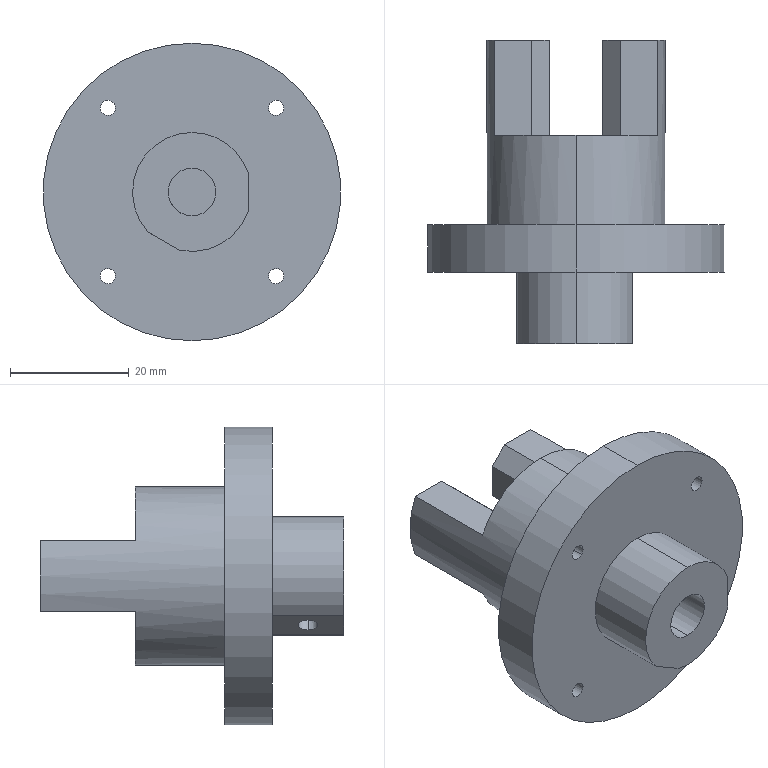Part | NX | features BREP 1 | 1 solid | 44 faces | box 50 x 51 x 50 mm | volume 32807 mm3 | cylinder 25 | plane 19 | commonest cylinder face diameters 2.5 x12 3.3 x4 20 x3 8 x2 30 x2 50 x2
STEP:
#1=CARTESIAN_POINT('',(14.122,12.,15.412));
#2=VERTEX_POINT('',#1);
#3=CARTESIAN_POINT('',(15.026,12.,15.026));
#4=VERTEX_POINT('',#3);
#5=CARTESIAN_POINT('',(14.122,12.,14.162));
#6=DIRECTION('',(0.,1.,0.));
#7=DIRECTION('',(0.,0.,1.));
#8=AXIS2_PLACEMENT_3D('',#5,#6,#7);
#9=CIRCLE('',#8,1.25);
#10=EDGE_CURVE('',#2,#4,#9,.T.);
#11=ORIENTED_EDGE('',*,*,#10,.F.);
#12=CARTESIAN_POINT('',(14.122,20.,15.412));
#13=VERTEX_POINT('',#12);
#14=CARTESIAN_POINT('',(14.122,20.,15.412));
#15=DIRECTION('',(0.,1.,0.));
#16=VECTOR('',#15,1000.);
#17=LINE('',#14,#16);
#18=EDGE_CURVE('',#2,#13,#17,.T.);
#19=ORIENTED_EDGE('',*,*,#18,.T.);
#20=CARTESIAN_POINT('',(15.026,20.,15.026));
#21=VERTEX_POINT('',#20);
#22=CARTESIAN_POINT('',(14.122,20.,14.162));
#23=DIRECTION('',(0.,1.,0.));
#24=DIRECTION('',(0.,0.,1.));
#25=AXIS2_PLACEMENT_3D('',#22,#23,#24);
#26=CIRCLE('',#25,1.25);
#27=EDGE_CURVE('',#13,#21,#26,.T.);
#28=ORIENTED_EDGE('',*,*,#27,.T.);
#29=CARTESIAN_POINT('',(15.026,15.75,15.026));
#30=DIRECTION('',(0.,1.,0.));
#31=VECTOR('',#30,1000.);
#32=LINE('',#29,#31);
#33=EDGE_CURVE('',#4,#21,#32,.T.);
#34=ORIENTED_EDGE('',*,*,#33,.F.);
#35=EDGE_LOOP('',(#11,#19,#28,#34));
#36=FACE_BOUND('',#35,.T.);
#37=CARTESIAN_POINT('',(14.122,20.,14.162));
#38=DIRECTION('',(0.,1.,0.));
#39=DIRECTION('',(0.,0.,-1.));
#40=AXIS2_PLACEMENT_3D('',#37,#38,#39);
#41=CYLINDRICAL_SURFACE('',#40,1.25);
#42=ADVANCED_FACE('',(#36),#41,.F.);
#43=CARTESIAN_POINT('',(-14.162,12.,-12.872));
#44=VERTEX_POINT('',#43);
#45=CARTESIAN_POINT('',(-13.258,12.,-13.258));
#46=VERTEX_POINT('',#45);
#47=CARTESIAN_POINT('',(-14.162,12.,-14.122));
#48=DIRECTION('',(0.,1.,0.));
#49=DIRECTION('',(0.,0.,1.));
#50=AXIS2_PLACEMENT_3D('',#47,#48,#49);
#51=CIRCLE('',#50,1.25);
#52=EDGE_CURVE('',#44,#46,#51,.T.);
#53=ORIENTED_EDGE('',*,*,#52,.F.);
#54=CARTESIAN_POINT('',(-14.162,20.,-12.872));
#55=VERTEX_POINT('',#54);
#56=CARTESIAN_POINT('',(-14.162,20.,-12.872));
#57=DIRECTION('',(0.,1.,0.));
#58=VECTOR('',#57,1000.);
#59=LINE('',#56,#58);
#60=EDGE_CURVE('',#44,#55,#59,.T.);
#61=ORIENTED_EDGE('',*,*,#60,.T.);
#62=CARTESIAN_POINT('',(-13.258,20.,-13.258));
#63=VERTEX_POINT('',#62);
#64=CARTESIAN_POINT('',(-14.162,20.,-14.122));
#65=DIRECTION('',(0.,1.,0.));
#66=DIRECTION('',(0.,0.,1.));
#67=AXIS2_PLACEMENT_3D('',#64,#65,#66);
#68=CIRCLE('',#67,1.25);
#69=EDGE_CURVE('',#55,#63,#68,.T.);
#70=ORIENTED_EDGE('',*,*,#69,.T.);
#71=CARTESIAN_POINT('',(-13.258,15.75,-13.258));
#72=DIRECTION('',(0.,1.,0.));
#73=VECTOR('',#72,1000.);
#74=LINE('',#71,#73);
#75=EDGE_CURVE('',#46,#63,#74,.T.);
#76=ORIENTED_EDGE('',*,*,#75,.F.);
#77=EDGE_LOOP('',(#53,#61,#70,#76));
#78=FACE_BOUND('',#77,.T.);
#79=CARTESIAN_POINT('',(-14.162,20.,-14.122));
#80=DIRECTION('',(0.,1.,0.));
#81=DIRECTION('',(0.,0.,-1.));
#82=AXIS2_PLACEMENT_3D('',#79,#80,#81);
#83=CYLINDRICAL_SURFACE('',#82,1.25);
#84=ADVANCED_FACE('',(#78),#83,.F.);
#85=CARTESIAN_POINT('',(14.162,12.,-12.872));
#86=VERTEX_POINT('',#85);
#87=CARTESIAN_POINT('',(15.026,12.,-15.026));
#88=VERTEX_POINT('',#87);
#89=CARTESIAN_POINT('',(14.162,12.,-14.122));
#90=DIRECTION('',(0.,1.,0.));
#91=DIRECTION('',(0.,0.,1.));
#92=AXIS2_PLACEMENT_3D('',#89,#90,#91);
#93=CIRCLE('',#92,1.25);
#94=EDGE_CURVE('',#86,#88,#93,.T.);
#95=ORIENTED_EDGE('',*,*,#94,.F.);
#96=CARTESIAN_POINT('',(14.162,20.,-12.872));
#97=VERTEX_POINT('',#96);
#98=CARTESIAN_POINT('',(14.162,20.,-12.872));
#99=DIRECTION('',(0.,1.,0.));
#100=VECTOR('',#99,1000.);
#101=LINE('',#98,#100);
#102=EDGE_CURVE('',#86,#97,#101,.T.);
#103=ORIENTED_EDGE('',*,*,#102,.T.);
#104=CARTESIAN_POINT('',(15.026,20.,-15.026));
#105=VERTEX_POINT('',#104);
#106=CARTESIAN_POINT('',(14.162,20.,-14.122));
#107=DIRECTION('',(0.,1.,0.));
#108=DIRECTION('',(0.,0.,1.));
#109=AXIS2_PLACEMENT_3D('',#106,#107,#108);
#110=CIRCLE('',#109,1.25);
#111=EDGE_CURVE('',#97,#105,#110,.T.);
#112=ORIENTED_EDGE('',*,*,#111,.T.);
#113=CARTESIAN_POINT('',(15.026,15.75,-15.026));
#114=DIRECTION('',(0.,-1.,0.));
#115=VECTOR('',#114,1000.);
#116=LINE('',#113,#115);
#117=EDGE_CURVE('',#105,#88,#116,.T.);
#118=ORIENTED_EDGE('',*,*,#117,.T.);
#119=EDGE_LOOP('',(#95,#103,#112,#118));
#120=FACE_BOUND('',#119,.T.);
#121=CARTESIAN_POINT('',(14.162,20.,-14.122));
#122=DIRECTION('',(0.,1.,0.));
#123=DIRECTION('',(0.,0.,-1.));
#124=AXIS2_PLACEMENT_3D('',#121,#122,#123);
#125=CYLINDRICAL_SURFACE('',#124,1.25);
#126=ADVANCED_FACE('',(#120),#125,.F.);
#127=CARTESIAN_POINT('',(-14.122,12.,15.412));
#128=VERTEX_POINT('',#127);
#129=CARTESIAN_POINT('',(-13.258,12.,13.258));
#130=VERTEX_POINT('',#129);
#131=CARTESIAN_POINT('',(-14.122,12.,14.162));
#132=DIRECTION('',(0.,1.,0.));
#133=DIRECTION('',(0.,0.,1.));
#134=AXIS2_PLACEMENT_3D('',#131,#132,#133);
#135=CIRCLE('',#134,1.25);
#136=EDGE_CURVE('',#128,#130,#135,.T.);
#137=ORIENTED_EDGE('',*,*,#136,.F.);
#138=CARTESIAN_POINT('',(-14.122,20.,15.412));
#139=VERTEX_POINT('',#138);
#140=CARTESIAN_POINT('',(-14.122,20.,15.412));
#141=DIRECTION('',(0.,1.,0.));
#142=VECTOR('',#141,1000.);
#143=LINE('',#140,#142);
#144=EDGE_CURVE('',#128,#139,#143,.T.);
#145=ORIENTED_EDGE('',*,*,#144,.T.);
#146=CARTESIAN_POINT('',(-13.258,20.,13.258));
#147=VERTEX_POINT('',#146);
#148=CARTESIAN_POINT('',(-14.122,20.,14.162));
#149=DIRECTION('',(0.,1.,0.));
#150=DIRECTION('',(0.,0.,1.));
#151=AXIS2_PLACEMENT_3D('',#148,#149,#150);
#152=CIRCLE('',#151,1.25);
#153=EDGE_CURVE('',#139,#147,#152,.T.);
#154=ORIENTED_EDGE('',*,*,#153,.T.);
#155=CARTESIAN_POINT('',(-13.258,15.75,13.258));
#156=DIRECTION('',(0.,1.,0.));
#157=VECTOR('',#156,1000.);
#158=LINE('',#155,#157);
#159=EDGE_CURVE('',#130,#147,#158,.T.);
#160=ORIENTED_EDGE('',*,*,#159,.F.);
#161=EDGE_LOOP('',(#137,#145,#154,#160));
#162=FACE_BOUND('',#161,.T.);
#163=CARTESIAN_POINT('',(-14.122,20.,14.162));
#164=DIRECTION('',(0.,1.,0.));
#165=DIRECTION('',(0.,0.,-1.));
#166=AXIS2_PLACEMENT_3D('',#163,#164,#165);
#167=CYLINDRICAL_SURFACE('',#166,1.25);
#168=ADVANCED_FACE('',(#162),#167,.F.);
#169=CARTESIAN_POINT('',(0.,20.,-15.));
#170=VERTEX_POINT('',#169);
#171=CARTESIAN_POINT('',(0.,20.,15.));
#172=VERTEX_POINT('',#171);
#173=CARTESIAN_POINT('',(0.,20.,0.));
#174=DIRECTION('',(0.,-1.,0.));
#175=DIRECTION('',(0.,0.,-1.));
#176=AXIS2_PLACEMENT_3D('',#173,#174,#175);
#177=CIRCLE('',#176,15.);
#178=EDGE_CURVE('',#170,#172,#177,.T.);
#179=ORIENTED_EDGE('',*,*,#178,.F.);
#180=CARTESIAN_POINT('',(0.,35.,-15.));
#181=VERTEX_POINT('',#180);
#182=CARTESIAN_POINT('',(0.,81.449,-15.));
#183=DIRECTION('',(0.,1.,0.));
#184=VECTOR('',#183,1000.);
#185=LINE('',#182,#184);
#186=EDGE_CURVE('',#170,#181,#185,.T.);
#187=ORIENTED_EDGE('',*,*,#186,.T.);
#188=CARTESIAN_POINT('',(13.748,35.,-6.));
#189=VERTEX_POINT('',#188);
#190=CARTESIAN_POINT('',(0.,35.,0.));
#191=DIRECTION('',(0.,1.,0.));
#192=DIRECTION('',(0.,0.,1.));
#193=AXIS2_PLACEMENT_3D('',#190,#191,#192);
#194=CIRCLE('',#193,15.);
#195=EDGE_CURVE('',#189,#181,#194,.T.);
#196=ORIENTED_EDGE('',*,*,#195,.F.);
#197=CARTESIAN_POINT('',(13.748,51.,-6.));
#198=VERTEX_POINT('',#197);
#199=CARTESIAN_POINT('',(13.748,81.449,-6.));
#200=DIRECTION('',(0.,1.,0.));
#201=VECTOR('',#200,1000.);
#202=LINE('',#199,#201);
#203=EDGE_CURVE('',#189,#198,#202,.T.);
#204=ORIENTED_EDGE('',*,*,#203,.T.);
#205=CARTESIAN_POINT('',(13.748,51.,6.));
#206=VERTEX_POINT('',#205);
#207=CARTESIAN_POINT('',(0.,51.,0.));
#208=DIRECTION('',(0.,1.,0.));
#209=DIRECTION('',(0.,0.,1.));
#210=AXIS2_PLACEMENT_3D('',#207,#208,#209);
#211=CIRCLE('',#210,15.);
#212=EDGE_CURVE('',#206,#198,#211,.T.);
#213=ORIENTED_EDGE('',*,*,#212,.F.);
#214=CARTESIAN_POINT('',(13.748,35.,6.));
#215=VERTEX_POINT('',#214);
#216=CARTESIAN_POINT('',(13.748,81.449,6.));
#217=DIRECTION('',(0.,-1.,0.));
#218=VECTOR('',#217,1000.);
#219=LINE('',#216,#218);
#220=EDGE_CURVE('',#206,#215,#219,.T.);
#221=ORIENTED_EDGE('',*,*,#220,.T.);
#222=CARTESIAN_POINT('',(0.,35.,15.));
#223=VERTEX_POINT('',#222);
#224=CARTESIAN_POINT('',(0.,35.,0.));
#225=DIRECTION('',(0.,1.,0.));
#226=DIRECTION('',(0.,0.,1.));
#227=AXIS2_PLACEMENT_3D('',#224,#225,#226);
#228=CIRCLE('',#227,15.);
#229=EDGE_CURVE('',#223,#215,#228,.T.);
#230=ORIENTED_EDGE('',*,*,#229,.F.);
#231=CARTESIAN_POINT('',(0.,81.449,15.));
#232=DIRECTION('',(0.,1.,0.));
#233=VECTOR('',#232,1000.);
#234=LINE('',#231,#233);
#235=EDGE_CURVE('',#172,#223,#234,.T.);
#236=ORIENTED_EDGE('',*,*,#235,.F.);
#237=EDGE_LOOP('',(#179,#187,#196,#204,#213,#221,#230,#236));
#238=FACE_BOUND('',#237,.T.);
#239=CARTESIAN_POINT('',(0.,81.449,0.));
#240=DIRECTION('',(0.,1.,0.));
#241=DIRECTION('',(0.,0.,-1.));
#242=AXIS2_PLACEMENT_3D('',#239,#240,#241);
#243=CYLINDRICAL_SURFACE('',#242,15.);
#244=ADVANCED_FACE('',(#238),#243,.T.);
#245=CARTESIAN_POINT('',(0.,20.,-25.));
#246=VERTEX_POINT('',#245);
#247=CARTESIAN_POINT('',(0.,20.,25.));
#248=VERTEX_POINT('',#247);
#249=CARTESIAN_POINT('',(0.,20.,0.));
#250=DIRECTION('',(0.,-1.,0.));
#251=DIRECTION('',(0.,0.,-1.));
#252=AXIS2_PLACEMENT_3D('',#249,#250,#251);
#253=CIRCLE('',#252,25.);
#254=EDGE_CURVE('',#246,#248,#253,.T.);
#255=ORIENTED_EDGE('',*,*,#254,.T.);
#256=CARTESIAN_POINT('',(0.,12.,25.));
#257=VERTEX_POINT('',#256);
#258=CARTESIAN_POINT('',(0.,20.,25.));
#259=DIRECTION('',(0.,-1.,0.));
#260=VECTOR('',#259,1000.);
#261=LINE('',#258,#260);
#262=EDGE_CURVE('',#257,#248,#261,.F.);
#263=ORIENTED_EDGE('',*,*,#262,.F.);
#264=CARTESIAN_POINT('',(0.,12.,-25.));
#265=VERTEX_POINT('',#264);
#266=CARTESIAN_POINT('',(0.,12.,0.));
#267=DIRECTION('',(0.,-1.,0.));
#268=DIRECTION('',(0.,0.,-1.));
#269=AXIS2_PLACEMENT_3D('',#266,#267,#268);
#270=CIRCLE('',#269,25.);
#271=EDGE_CURVE('',#265,#257,#270,.T.);
#272=ORIENTED_EDGE('',*,*,#271,.F.);
#273=CARTESIAN_POINT('',(0.,20.,-25.));
#274=DIRECTION('',(0.,-1.,0.));
#275=VECTOR('',#274,1000.);
#276=LINE('',#273,#275);
#277=EDGE_CURVE('',#265,#246,#276,.F.);
#278=ORIENTED_EDGE('',*,*,#277,.T.);
#279=EDGE_LOOP('',(#255,#263,#272,#278));
#280=FACE_BOUND('',#279,.T.);
#281=CARTESIAN_POINT('',(0.,20.,0.));
#282=DIRECTION('',(0.,-1.,0.));
#283=DIRECTION('',(0.,0.,1.));
#284=AXIS2_PLACEMENT_3D('',#281,#282,#283);
#285=CYLINDRICAL_SURFACE('',#284,25.);
#286=ADVANCED_FACE('',(#280),#285,.T.);
#287=CARTESIAN_POINT('',(-0.393,6.,-3.981));
#288=VERTEX_POINT('',#287);
#289=CARTESIAN_POINT('',(-3.251,6.,-2.331));
#290=VERTEX_POINT('',#289);
#291=CARTESIAN_POINT('',(-0.393,6.,-3.981));
#292=CARTESIAN_POINT('',(-0.393,5.559,-3.981));
#293=CARTESIAN_POINT('',(-0.7955,4.713,-3.963));
#294=CARTESIAN_POINT('',(-2.039,4.169,-3.539));
#295=CARTESIAN_POINT('',(-3.036,4.712,-2.67));
#296=CARTESIAN_POINT('',(-3.251,5.559,-2.331));
#297=CARTESIAN_POINT('',(-3.251,6.,-2.331));
#298=B_SPLINE_CURVE_WITH_KNOTS('',3,(#291,#292,#293,#294,#295,#296,#297),.UNSPECIFIED.,.F.,.F.,(4,1,1,1,4),(0.,0.001304,0.002607,0.003911,0.005215),.UNSPECIFIED.);
#299=EDGE_CURVE('',#288,#290,#298,.T.);
#300=ORIENTED_EDGE('',*,*,#299,.F.);
#301=CARTESIAN_POINT('',(-3.321,6.,-9.052));
#302=VERTEX_POINT('',#301);
#303=CARTESIAN_POINT('',(-3.571,6.,-9.485));
#304=DIRECTION('',(-0.5,0.,-0.866));
#305=VECTOR('',#304,1000.);
#306=LINE('',#303,#305);
#307=EDGE_CURVE('',#302,#288,#306,.F.);
#308=ORIENTED_EDGE('',*,*,#307,.F.);
#309=CARTESIAN_POINT('',(-6.179,6.,-7.402));
#310=VERTEX_POINT('',#309);
#311=CARTESIAN_POINT('',(-4.75,6.,-8.227));
#312=DIRECTION('',(-0.5,0.,-0.866));
#313=DIRECTION('',(0.866,0.,-0.5));
#314=AXIS2_PLACEMENT_3D('',#311,#312,#313);
#315=CIRCLE('',#314,1.65);
#316=EDGE_CURVE('',#302,#310,#315,.T.);
#317=ORIENTED_EDGE('',*,*,#316,.T.);
#318=CARTESIAN_POINT('',(-6.429,6.,-7.835));
#319=DIRECTION('',(-0.5,0.,-0.866));
#320=VECTOR('',#319,1000.);
#321=LINE('',#318,#320);
#322=EDGE_CURVE('',#310,#290,#321,.F.);
#323=ORIENTED_EDGE('',*,*,#322,.T.);
#324=EDGE_LOOP('',(#300,#308,#317,#323));
#325=FACE_BOUND('',#324,.T.);
#326=CARTESIAN_POINT('',(-5.,6.,-8.66));
#327=DIRECTION('',(-0.5,0.,-0.866));
#328=DIRECTION('',(0.866,0.,-0.5));
#329=AXIS2_PLACEMENT_3D('',#326,#327,#328);
#330=CYLINDRICAL_SURFACE('',#329,1.65);
#331=ADVANCED_FACE('',(#325),#330,.F.);
#332=CARTESIAN_POINT('',(3.644,6.,1.65));
#333=VERTEX_POINT('',#332);
#334=CARTESIAN_POINT('',(3.644,6.,-1.65));
#335=VERTEX_POINT('',#334);
#336=CARTESIAN_POINT('',(3.644,6.,1.65));
#337=CARTESIAN_POINT('',(3.644,5.559,1.65));
#338=CARTESIAN_POINT('',(3.83,4.713,1.293));
#339=CARTESIAN_POINT('',(4.085,4.169,0.003454));
#340=CARTESIAN_POINT('',(3.83,4.712,-1.294));
#341=CARTESIAN_POINT('',(3.644,5.559,-1.65));
#342=CARTESIAN_POINT('',(3.644,6.,-1.65));
#343=B_SPLINE_CURVE_WITH_KNOTS('',3,(#336,#337,#338,#339,#340,#341,#342),.UNSPECIFIED.,.F.,.F.,(4,1,1,1,4),(0.,0.001304,0.002607,0.003911,0.005215),.UNSPECIFIED.);
#344=EDGE_CURVE('',#333,#335,#343,.T.);
#345=ORIENTED_EDGE('',*,*,#344,.F.);
#346=CARTESIAN_POINT('',(9.5,6.,1.65));
#347=VERTEX_POINT('',#346);
#348=CARTESIAN_POINT('',(10.,6.,1.65));
#349=DIRECTION('',(1.,0.,0.));
#350=VECTOR('',#349,1000.);
#351=LINE('',#348,#350);
#352=EDGE_CURVE('',#347,#333,#351,.F.);
#353=ORIENTED_EDGE('',*,*,#352,.F.);
#354=CARTESIAN_POINT('',(9.5,6.,-1.65));
#355=VERTEX_POINT('',#354);
#356=CARTESIAN_POINT('',(9.5,6.,0.));
#357=DIRECTION('',(1.,0.,0.));
#358=DIRECTION('',(0.,0.,1.));
#359=AXIS2_PLACEMENT_3D('',#356,#357,#358);
#360=CIRCLE('',#359,1.65);
#361=EDGE_CURVE('',#347,#355,#360,.T.);
#362=ORIENTED_EDGE('',*,*,#361,.T.);
#363=CARTESIAN_POINT('',(10.,6.,-1.65));
#364=DIRECTION('',(1.,0.,0.));
#365=VECTOR('',#364,1000.);
#366=LINE('',#363,#365);
#367=EDGE_CURVE('',#355,#335,#366,.F.);
#368=ORIENTED_EDGE('',*,*,#367,.T.);
#369=EDGE_LOOP('',(#345,#353,#362,#368));
#370=FACE_BOUND('',#369,.T.);
#371=CARTESIAN_POINT('',(10.,6.,0.));
#372=DIRECTION('',(1.,0.,0.));
#373=DIRECTION('',(0.,0.,1.));
#374=AXIS2_PLACEMENT_3D('',#371,#372,#373);
#375=CYLINDRICAL_SURFACE('',#374,1.65);
#376=ADVANCED_FACE('',(#370),#375,.F.);
#377=CARTESIAN_POINT('',(-3.251,6.,-2.331));
#378=CARTESIAN_POINT('',(-3.251,6.441,-2.331));
#379=CARTESIAN_POINT('',(-3.034,7.287,-2.671));
#380=CARTESIAN_POINT('',(-2.045,7.831,-3.536));
#381=CARTESIAN_POINT('',(-0.7946,7.288,-3.964));
#382=CARTESIAN_POINT('',(-0.393,6.441,-3.981));
#383=CARTESIAN_POINT('',(-0.393,6.,-3.981));
#384=B_SPLINE_CURVE_WITH_KNOTS('',3,(#377,#378,#379,#380,#381,#382,#383),.UNSPECIFIED.,.F.,.F.,(4,1,1,1,4),(0.,0.001304,0.002607,0.003911,0.005215),.UNSPECIFIED.);
#385=EDGE_CURVE('',#290,#288,#384,.T.);
#386=ORIENTED_EDGE('',*,*,#385,.T.);
#387=ORIENTED_EDGE('',*,*,#299,.T.);
#388=EDGE_LOOP('',(#386,#387));
#389=FACE_BOUND('',#388,.T.);
#390=CARTESIAN_POINT('',(0.,11.,4.));
#391=VERTEX_POINT('',#390);
#392=CARTESIAN_POINT('',(0.,11.,-4.));
#393=VERTEX_POINT('',#392);
#394=CARTESIAN_POINT('',(0.,11.,0.));
#395=DIRECTION('',(0.,-1.,0.));
#396=DIRECTION('',(0.,0.,-1.));
#397=AXIS2_PLACEMENT_3D('',#394,#395,#396);
#398=CIRCLE('',#397,4.);
#399=EDGE_CURVE('',#391,#393,#398,.T.);
#400=ORIENTED_EDGE('',*,*,#399,.F.);
#401=CARTESIAN_POINT('',(0.,0.,4.));
#402=VERTEX_POINT('',#401);
#403=CARTESIAN_POINT('',(0.,11.,4.));
#404=DIRECTION('',(0.,-1.,0.));
#405=VECTOR('',#404,1000.);
#406=LINE('',#403,#405);
#407=EDGE_CURVE('',#402,#391,#406,.F.);
#408=ORIENTED_EDGE('',*,*,#407,.F.);
#409=CARTESIAN_POINT('',(0.,0.,-4.));
#410=VERTEX_POINT('',#409);
#411=CARTESIAN_POINT('',(0.,0.,0.));
#412=DIRECTION('',(0.,-1.,0.));
#413=DIRECTION('',(0.,0.,-1.));
#414=AXIS2_PLACEMENT_3D('',#411,#412,#413);
#415=CIRCLE('',#414,4.);
#416=EDGE_CURVE('',#402,#410,#415,.T.);
#417=ORIENTED_EDGE('',*,*,#416,.T.);
#418=CARTESIAN_POINT('',(0.,11.,-4.));
#419=DIRECTION('',(0.,-1.,0.));
#420=VECTOR('',#419,1000.);
#421=LINE('',#418,#420);
#422=EDGE_CURVE('',#410,#393,#421,.F.);
#423=ORIENTED_EDGE('',*,*,#422,.T.);
#424=EDGE_LOOP('',(#400,#408,#417,#423));
#425=FACE_BOUND('',#424,.T.);
#426=CARTESIAN_POINT('',(0.,11.,0.));
#427=DIRECTION('',(0.,-1.,0.));
#428=DIRECTION('',(0.,0.,1.));
#429=AXIS2_PLACEMENT_3D('',#426,#427,#428);
#430=CYLINDRICAL_SURFACE('',#429,4.);
#431=ADVANCED_FACE('',(#389,#425),#430,.F.);
#432=CARTESIAN_POINT('',(-7.454,0.,-6.666));
#433=VERTEX_POINT('',#432);
#434=CARTESIAN_POINT('',(0.,0.,10.));
#435=VERTEX_POINT('',#434);
#436=CARTESIAN_POINT('',(0.,0.,0.));
#437=DIRECTION('',(0.,1.,0.));
#438=DIRECTION('',(0.,0.,1.));
#439=AXIS2_PLACEMENT_3D('',#436,#437,#438);
#440=CIRCLE('',#439,10.);
#441=EDGE_CURVE('',#433,#435,#440,.T.);
#442=ORIENTED_EDGE('',*,*,#441,.T.);
#443=CARTESIAN_POINT('',(0.,12.,10.));
#444=VERTEX_POINT('',#443);
#445=CARTESIAN_POINT('',(0.,81.449,10.));
#446=DIRECTION('',(0.,1.,0.));
#447=VECTOR('',#446,1000.);
#448=LINE('',#445,#447);
#449=EDGE_CURVE('',#435,#444,#448,.T.);
#450=ORIENTED_EDGE('',*,*,#449,.T.);
#451=CARTESIAN_POINT('',(-7.454,12.,-6.666));
#452=VERTEX_POINT('',#451);
#453=CARTESIAN_POINT('',(0.,12.,0.));
#454=DIRECTION('',(0.,1.,0.));
#455=DIRECTION('',(0.,0.,1.));
#456=AXIS2_PLACEMENT_3D('',#453,#454,#455);
#457=CIRCLE('',#456,10.);
#458=EDGE_CURVE('',#452,#444,#457,.T.);
#459=ORIENTED_EDGE('',*,*,#458,.F.);
#460=CARTESIAN_POINT('',(-7.454,18.245,-6.666));
#461=DIRECTION('',(0.,-1.,0.));
#462=VECTOR('',#461,1000.);
#463=LINE('',#460,#462);
#464=EDGE_CURVE('',#452,#433,#463,.T.);
#465=ORIENTED_EDGE('',*,*,#464,.T.);
#466=EDGE_LOOP('',(#442,#450,#459,#465));
#467=FACE_BOUND('',#466,.T.);
#468=CARTESIAN_POINT('',(0.,81.449,0.));
#469=DIRECTION('',(0.,1.,0.));
#470=DIRECTION('',(0.,0.,-1.));
#471=AXIS2_PLACEMENT_3D('',#468,#469,#470);
#472=CYLINDRICAL_SURFACE('',#471,10.);
#473=ADVANCED_FACE('',(#467),#472,.T.);
#474=CARTESIAN_POINT('',(13.258,20.,13.258));
#475=VERTEX_POINT('',#474);
#476=CARTESIAN_POINT('',(14.122,20.,14.162));
#477=DIRECTION('',(0.,1.,0.));
#478=DIRECTION('',(0.,0.,1.));
#479=AXIS2_PLACEMENT_3D('',#476,#477,#478);
#480=CIRCLE('',#479,1.25);
#481=EDGE_CURVE('',#475,#13,#480,.T.);
#482=ORIENTED_EDGE('',*,*,#481,.F.);
#483=CARTESIAN_POINT('',(14.162,20.,14.122));
#484=DIRECTION('',(0.,1.,0.));
#485=DIRECTION('',(0.,0.,1.));
#486=AXIS2_PLACEMENT_3D('',#483,#484,#485);
#487=CIRCLE('',#486,1.25);
#488=EDGE_CURVE('',#21,#475,#487,.T.);
#489=ORIENTED_EDGE('',*,*,#488,.F.);
#490=ORIENTED_EDGE('',*,*,#27,.F.);
#491=EDGE_LOOP('',(#482,#489,#490));
#492=FACE_BOUND('',#491,.T.);
#493=CARTESIAN_POINT('',(-15.026,20.,15.026));
#494=VERTEX_POINT('',#493);
#495=CARTESIAN_POINT('',(-14.122,20.,14.162));
#496=DIRECTION('',(0.,1.,0.));
#497=DIRECTION('',(0.,0.,1.));
#498=AXIS2_PLACEMENT_3D('',#495,#496,#497);
#499=CIRCLE('',#498,1.25);
#500=EDGE_CURVE('',#494,#139,#499,.T.);
#501=ORIENTED_EDGE('',*,*,#500,.F.);
#502=CARTESIAN_POINT('',(-14.162,20.,14.122));
#503=DIRECTION('',(0.,1.,0.));
#504=DIRECTION('',(0.,0.,1.));
#505=AXIS2_PLACEMENT_3D('',#502,#503,#504);
#506=CIRCLE('',#505,1.25);
#507=EDGE_CURVE('',#147,#494,#506,.T.);
#508=ORIENTED_EDGE('',*,*,#507,.F.);
#509=ORIENTED_EDGE('',*,*,#153,.F.);
#510=EDGE_LOOP('',(#501,#508,#509));
#511=FACE_BOUND('',#510,.T.);
#512=CARTESIAN_POINT('',(0.,20.,0.));
#513=DIRECTION('',(0.,-1.,0.));
#514=DIRECTION('',(0.,0.,-1.));
#515=AXIS2_PLACEMENT_3D('',#512,#513,#514);
#516=CIRCLE('',#515,15.);
#517=EDGE_CURVE('',#172,#170,#516,.T.);
#518=ORIENTED_EDGE('',*,*,#517,.T.);
#519=ORIENTED_EDGE('',*,*,#178,.T.);
#520=EDGE_LOOP('',(#518,#519));
#521=FACE_BOUND('',#520,.T.);
#522=ORIENTED_EDGE('',*,*,#254,.F.);
#523=CARTESIAN_POINT('',(0.,20.,0.));
#524=DIRECTION('',(0.,-1.,0.));
#525=DIRECTION('',(0.,0.,-1.));
#526=AXIS2_PLACEMENT_3D('',#523,#524,#525);
#527=CIRCLE('',#526,25.);
#528=EDGE_CURVE('',#248,#246,#527,.T.);
#529=ORIENTED_EDGE('',*,*,#528,.F.);
#530=EDGE_LOOP('',(#522,#529));
#531=FACE_BOUND('',#530,.T.);
#532=CARTESIAN_POINT('',(-15.026,20.,-15.026));
#533=VERTEX_POINT('',#532);
#534=CARTESIAN_POINT('',(-14.162,20.,-14.122));
#535=DIRECTION('',(0.,1.,0.));
#536=DIRECTION('',(0.,0.,1.));
#537=AXIS2_PLACEMENT_3D('',#534,#535,#536);
#538=CIRCLE('',#537,1.25);
#539=EDGE_CURVE('',#533,#55,#538,.T.);
#540=ORIENTED_EDGE('',*,*,#539,.F.);
#541=CARTESIAN_POINT('',(-14.122,20.,-14.162));
#542=DIRECTION('',(0.,1.,0.));
#543=DIRECTION('',(0.,0.,1.));
#544=AXIS2_PLACEMENT_3D('',#541,#542,#543);
#545=CIRCLE('',#544,1.25);
#546=EDGE_CURVE('',#63,#533,#545,.T.);
#547=ORIENTED_EDGE('',*,*,#546,.F.);
#548=ORIENTED_EDGE('',*,*,#69,.F.);
#549=EDGE_LOOP('',(#540,#547,#548));
#550=FACE_BOUND('',#549,.T.);
#551=CARTESIAN_POINT('',(13.258,20.,-13.258));
#552=VERTEX_POINT('',#551);
#553=CARTESIAN_POINT('',(14.122,20.,-14.162));
#554=DIRECTION('',(0.,1.,0.));
#555=DIRECTION('',(0.,0.,1.));
#556=AXIS2_PLACEMENT_3D('',#553,#554,#555);
#557=CIRCLE('',#556,1.25);
#558=EDGE_CURVE('',#105,#552,#557,.T.);
#559=ORIENTED_EDGE('',*,*,#558,.F.);
#560=ORIENTED_EDGE('',*,*,#111,.F.);
#561=CARTESIAN_POINT('',(14.162,20.,-14.122));
#562=DIRECTION('',(0.,1.,0.));
#563=DIRECTION('',(0.,0.,1.));
#564=AXIS2_PLACEMENT_3D('',#561,#562,#563);
#565=CIRCLE('',#564,1.25);
#566=EDGE_CURVE('',#552,#97,#565,.T.);
#567=ORIENTED_EDGE('',*,*,#566,.F.);
#568=EDGE_LOOP('',(#559,#560,#567));
#569=FACE_BOUND('',#568,.T.);
#570=CARTESIAN_POINT('',(0.,20.,0.));
#571=DIRECTION('',(0.,-1.,0.));
#572=DIRECTION('',(0.,0.,1.));
#573=AXIS2_PLACEMENT_3D('',#570,#571,#572);
#574=PLANE('',#573);
#575=ADVANCED_FACE('',(#492,#511,#521,#531,#550,#569),#574,.F.);
#576=CARTESIAN_POINT('',(9.5,0.,-3.122));
#577=VERTEX_POINT('',#576);
#578=CARTESIAN_POINT('',(-2.046,0.,-9.788));
#579=VERTEX_POINT('',#578);
#580=CARTESIAN_POINT('',(0.,0.,0.));
#581=DIRECTION('',(0.,1.,0.));
#582=DIRECTION('',(0.,0.,1.));
#583=AXIS2_PLACEMENT_3D('',#580,#581,#582);
#584=CIRCLE('',#583,10.);
#585=EDGE_CURVE('',#577,#579,#584,.T.);
#586=ORIENTED_EDGE('',*,*,#585,.T.);
#587=CARTESIAN_POINT('',(-2.046,12.,-9.788));
#588=VERTEX_POINT('',#587);
#589=CARTESIAN_POINT('',(-2.046,18.245,-9.788));
#590=DIRECTION('',(0.,-1.,0.));
#591=VECTOR('',#590,1000.);
#592=LINE('',#589,#591);
#593=EDGE_CURVE('',#588,#579,#592,.T.);
#594=ORIENTED_EDGE('',*,*,#593,.F.);
#595=CARTESIAN_POINT('',(9.5,12.,-3.122));
#596=VERTEX_POINT('',#595);
#597=CARTESIAN_POINT('',(0.,12.,0.));
#598=DIRECTION('',(0.,1.,0.));
#599=DIRECTION('',(0.,0.,1.));
#600=AXIS2_PLACEMENT_3D('',#597,#598,#599);
#601=CIRCLE('',#600,10.);
#602=EDGE_CURVE('',#596,#588,#601,.T.);
#603=ORIENTED_EDGE('',*,*,#602,.F.);
#604=CARTESIAN_POINT('',(9.5,18.265,-3.122));
#605=DIRECTION('',(0.,-1.,0.));
#606=VECTOR('',#605,1000.);
#607=LINE('',#604,#606);
#608=EDGE_CURVE('',#596,#577,#607,.T.);
#609=ORIENTED_EDGE('',*,*,#608,.T.);
#610=EDGE_LOOP('',(#586,#594,#603,#609));
#611=FACE_BOUND('',#610,.T.);
#612=CARTESIAN_POINT('',(0.,81.449,0.));
#613=DIRECTION('',(0.,1.,0.));
#614=DIRECTION('',(0.,0.,-1.));
#615=AXIS2_PLACEMENT_3D('',#612,#613,#614);
#616=CYLINDRICAL_SURFACE('',#615,10.);
#617=ADVANCED_FACE('',(#611),#616,.T.);
#618=CARTESIAN_POINT('',(13.258,12.,-13.258));
#619=VERTEX_POINT('',#618);
#620=CARTESIAN_POINT('',(14.162,12.,-14.122));
#621=DIRECTION('',(0.,1.,0.));
#622=DIRECTION('',(0.,0.,1.));
#623=AXIS2_PLACEMENT_3D('',#620,#621,#622);
#624=CIRCLE('',#623,1.25);
#625=EDGE_CURVE('',#619,#86,#624,.T.);
#626=ORIENTED_EDGE('',*,*,#625,.T.);
#627=ORIENTED_EDGE('',*,*,#94,.T.);
#628=CARTESIAN_POINT('',(14.122,12.,-14.162));
#629=DIRECTION('',(0.,1.,0.));
#630=DIRECTION('',(0.,0.,1.));
#631=AXIS2_PLACEMENT_3D('',#628,#629,#630);
#632=CIRCLE('',#631,1.25);
#633=EDGE_CURVE('',#88,#619,#632,.T.);
#634=ORIENTED_EDGE('',*,*,#633,.T.);
#635=EDGE_LOOP('',(#626,#627,#634));
#636=FACE_BOUND('',#635,.T.);
#637=CARTESIAN_POINT('',(-15.026,12.,-15.026));
#638=VERTEX_POINT('',#637);
#639=CARTESIAN_POINT('',(-14.122,12.,-14.162));
#640=DIRECTION('',(0.,1.,0.));
#641=DIRECTION('',(0.,0.,1.));
#642=AXIS2_PLACEMENT_3D('',#639,#640,#641);
#643=CIRCLE('',#642,1.25);
#644=EDGE_CURVE('',#46,#638,#643,.T.);
#645=ORIENTED_EDGE('',*,*,#644,.T.);
#646=CARTESIAN_POINT('',(-14.162,12.,-14.122));
#647=DIRECTION('',(0.,1.,0.));
#648=DIRECTION('',(0.,0.,1.));
#649=AXIS2_PLACEMENT_3D('',#646,#647,#648);
#650=CIRCLE('',#649,1.25);
#651=EDGE_CURVE('',#638,#44,#650,.T.);
#652=ORIENTED_EDGE('',*,*,#651,.T.);
#653=ORIENTED_EDGE('',*,*,#52,.T.);
#654=EDGE_LOOP('',(#645,#652,#653));
#655=FACE_BOUND('',#654,.T.);
#656=CARTESIAN_POINT('',(13.258,12.,13.258));
#657=VERTEX_POINT('',#656);
#658=CARTESIAN_POINT('',(14.162,12.,14.122));
#659=DIRECTION('',(0.,1.,0.));
#660=DIRECTION('',(0.,0.,1.));
#661=AXIS2_PLACEMENT_3D('',#658,#659,#660);
#662=CIRCLE('',#661,1.25);
#663=EDGE_CURVE('',#4,#657,#662,.T.);
#664=ORIENTED_EDGE('',*,*,#663,.T.);
#665=CARTESIAN_POINT('',(14.122,12.,14.162));
#666=DIRECTION('',(0.,1.,0.));
#667=DIRECTION('',(0.,0.,1.));
#668=AXIS2_PLACEMENT_3D('',#665,#666,#667);
#669=CIRCLE('',#668,1.25);
#670=EDGE_CURVE('',#657,#2,#669,.T.);
#671=ORIENTED_EDGE('',*,*,#670,.T.);
#672=ORIENTED_EDGE('',*,*,#10,.T.);
#673=EDGE_LOOP('',(#664,#671,#672));
#674=FACE_BOUND('',#673,.T.);
#675=CARTESIAN_POINT('',(-15.026,12.,15.026));
#676=VERTEX_POINT('',#675);
#677=CARTESIAN_POINT('',(-14.162,12.,14.122));
#678=DIRECTION('',(0.,1.,0.));
#679=DIRECTION('',(0.,0.,1.));
#680=AXIS2_PLACEMENT_3D('',#677,#678,#679);
#681=CIRCLE('',#680,1.25);
#682=EDGE_CURVE('',#130,#676,#681,.T.);
#683=ORIENTED_EDGE('',*,*,#682,.T.);
#684=CARTESIAN_POINT('',(-14.122,12.,14.162));
#685=DIRECTION('',(0.,1.,0.));
#686=DIRECTION('',(0.,0.,1.));
#687=AXIS2_PLACEMENT_3D('',#684,#685,#686);
#688=CIRCLE('',#687,1.25);
#689=EDGE_CURVE('',#676,#128,#688,.T.);
#690=ORIENTED_EDGE('',*,*,#689,.T.);
#691=ORIENTED_EDGE('',*,*,#136,.T.);
#692=EDGE_LOOP('',(#683,#690,#691));
#693=FACE_BOUND('',#692,.T.);
#694=ORIENTED_EDGE('',*,*,#602,.T.);
#695=CARTESIAN_POINT('',(-2.046,12.,-9.788));
#696=DIRECTION('',(-0.866,0.,0.5));
#697=VECTOR('',#696,1000.);
#698=LINE('',#695,#697);
#699=EDGE_CURVE('',#588,#452,#698,.T.);
#700=ORIENTED_EDGE('',*,*,#699,.T.);
#701=ORIENTED_EDGE('',*,*,#458,.T.);
#702=CARTESIAN_POINT('',(9.5,12.,3.122));
#703=VERTEX_POINT('',#702);
#704=CARTESIAN_POINT('',(0.,12.,0.));
#705=DIRECTION('',(0.,1.,0.));
#706=DIRECTION('',(0.,0.,1.));
#707=AXIS2_PLACEMENT_3D('',#704,#705,#706);
#708=CIRCLE('',#707,10.);
#709=EDGE_CURVE('',#444,#703,#708,.T.);
#710=ORIENTED_EDGE('',*,*,#709,.T.);
#711=CARTESIAN_POINT('',(9.5,12.,3.122));
#712=DIRECTION('',(0.,0.,-1.));
#713=VECTOR('',#712,1000.);
#714=LINE('',#711,#713);
#715=EDGE_CURVE('',#703,#596,#714,.T.);
#716=ORIENTED_EDGE('',*,*,#715,.T.);
#717=EDGE_LOOP('',(#694,#700,#701,#710,#716));
#718=FACE_BOUND('',#717,.T.);
#719=ORIENTED_EDGE('',*,*,#271,.T.);
#720=CARTESIAN_POINT('',(0.,12.,0.));
#721=DIRECTION('',(0.,-1.,0.));
#722=DIRECTION('',(0.,0.,-1.));
#723=AXIS2_PLACEMENT_3D('',#720,#721,#722);
#724=CIRCLE('',#723,25.);
#725=EDGE_CURVE('',#257,#265,#724,.T.);
#726=ORIENTED_EDGE('',*,*,#725,.T.);
#727=EDGE_LOOP('',(#719,#726));
#728=FACE_BOUND('',#727,.T.);
#729=CARTESIAN_POINT('',(15.,12.,0.));
#730=DIRECTION('',(0.,1.,0.));
#731=DIRECTION('',(0.,0.,-1.));
#732=AXIS2_PLACEMENT_3D('',#729,#730,#731);
#733=PLANE('',#732);
#734=ADVANCED_FACE('',(#636,#655,#674,#693,#718,#728),#733,.F.);
#735=ORIENTED_EDGE('',*,*,#449,.F.);
#736=CARTESIAN_POINT('',(9.5,0.,3.122));
#737=VERTEX_POINT('',#736);
#738=CARTESIAN_POINT('',(0.,0.,0.));
#739=DIRECTION('',(0.,1.,0.));
#740=DIRECTION('',(0.,0.,1.));
#741=AXIS2_PLACEMENT_3D('',#738,#739,#740);
#742=CIRCLE('',#741,10.);
#743=EDGE_CURVE('',#435,#737,#742,.T.);
#744=ORIENTED_EDGE('',*,*,#743,.T.);
#745=CARTESIAN_POINT('',(9.5,18.265,3.122));
#746=DIRECTION('',(0.,-1.,0.));
#747=VECTOR('',#746,1000.);
#748=LINE('',#745,#747);
#749=EDGE_CURVE('',#703,#737,#748,.T.);
#750=ORIENTED_EDGE('',*,*,#749,.F.);
#751=ORIENTED_EDGE('',*,*,#709,.F.);
#752=EDGE_LOOP('',(#735,#744,#750,#751));
#753=FACE_BOUND('',#752,.T.);
#754=CARTESIAN_POINT('',(0.,81.449,0.));
#755=DIRECTION('',(0.,1.,0.));
#756=DIRECTION('',(0.,0.,-1.));
#757=AXIS2_PLACEMENT_3D('',#754,#755,#756);
#758=CYLINDRICAL_SURFACE('',#757,10.);
#759=ADVANCED_FACE('',(#753),#758,.T.);
#760=CARTESIAN_POINT('',(0.,0.,0.));
#761=DIRECTION('',(0.,-1.,0.));
#762=DIRECTION('',(0.,0.,-1.));
#763=AXIS2_PLACEMENT_3D('',#760,#761,#762);
#764=CIRCLE('',#763,4.);
#765=EDGE_CURVE('',#410,#402,#764,.T.);
#766=ORIENTED_EDGE('',*,*,#765,.F.);
#767=ORIENTED_EDGE('',*,*,#416,.F.);
#768=EDGE_LOOP('',(#766,#767));
#769=FACE_BOUND('',#768,.T.);
#770=ORIENTED_EDGE('',*,*,#441,.F.);
#771=CARTESIAN_POINT('',(-2.046,0.,-9.788));
#772=DIRECTION('',(-0.866,0.,0.5));
#773=VECTOR('',#772,1000.);
#774=LINE('',#771,#773);
#775=EDGE_CURVE('',#579,#433,#774,.T.);
#776=ORIENTED_EDGE('',*,*,#775,.F.);
#777=ORIENTED_EDGE('',*,*,#585,.F.);
#778=CARTESIAN_POINT('',(9.5,0.,3.122));
#779=DIRECTION('',(0.,0.,-1.));
#780=VECTOR('',#779,1000.);
#781=LINE('',#778,#780);
#782=EDGE_CURVE('',#737,#577,#781,.T.);
#783=ORIENTED_EDGE('',*,*,#782,.F.);
#784=ORIENTED_EDGE('',*,*,#743,.F.);
#785=EDGE_LOOP('',(#770,#776,#777,#783,#784));
#786=FACE_BOUND('',#785,.T.);
#787=CARTESIAN_POINT('',(10.,0.,0.));
#788=DIRECTION('',(0.,1.,0.));
#789=DIRECTION('',(0.,0.,-1.));
#790=AXIS2_PLACEMENT_3D('',#787,#788,#789);
#791=PLANE('',#790);
#792=ADVANCED_FACE('',(#769,#786),#791,.F.);
#793=ORIENTED_EDGE('',*,*,#407,.T.);
#794=CARTESIAN_POINT('',(0.,11.,0.));
#795=DIRECTION('',(0.,-1.,0.));
#796=DIRECTION('',(0.,0.,-1.));
#797=AXIS2_PLACEMENT_3D('',#794,#795,#796);
#798=CIRCLE('',#797,4.);
#799=EDGE_CURVE('',#393,#391,#798,.T.);
#800=ORIENTED_EDGE('',*,*,#799,.F.);
#801=ORIENTED_EDGE('',*,*,#422,.F.);
#802=ORIENTED_EDGE('',*,*,#765,.T.);
#803=EDGE_LOOP('',(#793,#800,#801,#802));
#804=FACE_BOUND('',#803,.T.);
#805=CARTESIAN_POINT('',(3.644,6.,-1.65));
#806=CARTESIAN_POINT('',(3.644,6.441,-1.65));
#807=CARTESIAN_POINT('',(3.83,7.287,-1.293));
#808=CARTESIAN_POINT('',(4.085,7.831,-0.003454));
#809=CARTESIAN_POINT('',(3.83,7.288,1.294));
#810=CARTESIAN_POINT('',(3.644,6.441,1.65));
#811=CARTESIAN_POINT('',(3.644,6.,1.65));
#812=B_SPLINE_CURVE_WITH_KNOTS('',3,(#805,#806,#807,#808,#809,#810,#811),.UNSPECIFIED.,.F.,.F.,(4,1,1,1,4),(0.,0.001304,0.002607,0.003911,0.005215),.UNSPECIFIED.);
#813=EDGE_CURVE('',#335,#333,#812,.T.);
#814=ORIENTED_EDGE('',*,*,#813,.T.);
#815=ORIENTED_EDGE('',*,*,#344,.T.);
#816=EDGE_LOOP('',(#814,#815));
#817=FACE_BOUND('',#816,.T.);
#818=CARTESIAN_POINT('',(0.,11.,0.));
#819=DIRECTION('',(0.,-1.,0.));
#820=DIRECTION('',(0.,0.,1.));
#821=AXIS2_PLACEMENT_3D('',#818,#819,#820);
#822=CYLINDRICAL_SURFACE('',#821,4.);
#823=ADVANCED_FACE('',(#804,#817),#822,.F.);
#824=ORIENTED_EDGE('',*,*,#799,.T.);
#825=ORIENTED_EDGE('',*,*,#399,.T.);
#826=EDGE_LOOP('',(#824,#825));
#827=FACE_BOUND('',#826,.T.);
#828=CARTESIAN_POINT('',(0.,11.,0.));
#829=DIRECTION('',(0.,-1.,0.));
#830=DIRECTION('',(0.,0.,1.));
#831=AXIS2_PLACEMENT_3D('',#828,#829,#830);
#832=PLANE('',#831);
#833=ADVANCED_FACE('',(#827),#832,.T.);
#834=ORIENTED_EDGE('',*,*,#352,.T.);
#835=ORIENTED_EDGE('',*,*,#813,.F.);
#836=ORIENTED_EDGE('',*,*,#367,.F.);
#837=CARTESIAN_POINT('',(9.5,6.,0.));
#838=DIRECTION('',(1.,0.,0.));
#839=DIRECTION('',(0.,0.,1.));
#840=AXIS2_PLACEMENT_3D('',#837,#838,#839);
#841=CIRCLE('',#840,1.65);
#842=EDGE_CURVE('',#355,#347,#841,.T.);
#843=ORIENTED_EDGE('',*,*,#842,.T.);
#844=EDGE_LOOP('',(#834,#835,#836,#843));
#845=FACE_BOUND('',#844,.T.);
#846=CARTESIAN_POINT('',(10.,6.,0.));
#847=DIRECTION('',(1.,0.,0.));
#848=DIRECTION('',(0.,0.,1.));
#849=AXIS2_PLACEMENT_3D('',#846,#847,#848);
#850=CYLINDRICAL_SURFACE('',#849,1.65);
#851=ADVANCED_FACE('',(#845),#850,.F.);
#852=ORIENTED_EDGE('',*,*,#749,.T.);
#853=ORIENTED_EDGE('',*,*,#782,.T.);
#854=ORIENTED_EDGE('',*,*,#608,.F.);
#855=ORIENTED_EDGE('',*,*,#715,.F.);
#856=EDGE_LOOP('',(#852,#853,#854,#855));
#857=FACE_BOUND('',#856,.T.);
#858=ORIENTED_EDGE('',*,*,#842,.F.);
#859=ORIENTED_EDGE('',*,*,#361,.F.);
#860=EDGE_LOOP('',(#858,#859));
#861=FACE_BOUND('',#860,.T.);
#862=CARTESIAN_POINT('',(9.5,18.265,3.122));
#863=DIRECTION('',(-1.,0.,0.));
#864=DIRECTION('',(0.,0.,-1.));
#865=AXIS2_PLACEMENT_3D('',#862,#863,#864);
#866=PLANE('',#865);
#867=ADVANCED_FACE('',(#857,#861),#866,.F.);
#868=ORIENTED_EDGE('',*,*,#307,.T.);
#869=ORIENTED_EDGE('',*,*,#385,.F.);
#870=ORIENTED_EDGE('',*,*,#322,.F.);
#871=CARTESIAN_POINT('',(-4.75,6.,-8.227));
#872=DIRECTION('',(-0.5,0.,-0.866));
#873=DIRECTION('',(0.866,0.,-0.5));
#874=AXIS2_PLACEMENT_3D('',#871,#872,#873);
#875=CIRCLE('',#874,1.65);
#876=EDGE_CURVE('',#310,#302,#875,.T.);
#877=ORIENTED_EDGE('',*,*,#876,.T.);
#878=EDGE_LOOP('',(#868,#869,#870,#877));
#879=FACE_BOUND('',#878,.T.);
#880=CARTESIAN_POINT('',(-5.,6.,-8.66));
#881=DIRECTION('',(-0.5,0.,-0.866));
#882=DIRECTION('',(0.866,0.,-0.5));
#883=AXIS2_PLACEMENT_3D('',#880,#881,#882);
#884=CYLINDRICAL_SURFACE('',#883,1.65);
#885=ADVANCED_FACE('',(#879),#884,.F.);
#886=ORIENTED_EDGE('',*,*,#593,.T.);
#887=ORIENTED_EDGE('',*,*,#775,.T.);
#888=ORIENTED_EDGE('',*,*,#464,.F.);
#889=ORIENTED_EDGE('',*,*,#699,.F.);
#890=EDGE_LOOP('',(#886,#887,#888,#889));
#891=FACE_BOUND('',#890,.T.);
#892=ORIENTED_EDGE('',*,*,#876,.F.);
#893=ORIENTED_EDGE('',*,*,#316,.F.);
#894=EDGE_LOOP('',(#892,#893));
#895=FACE_BOUND('',#894,.T.);
#896=CARTESIAN_POINT('',(-2.046,18.245,-9.788));
#897=DIRECTION('',(0.5,0.,0.866));
#898=DIRECTION('',(-0.866,0.,0.5));
#899=AXIS2_PLACEMENT_3D('',#896,#897,#898);
#900=PLANE('',#899);
#901=ADVANCED_FACE('',(#891,#895),#900,.F.);
#902=ORIENTED_EDGE('',*,*,#262,.T.);
#903=ORIENTED_EDGE('',*,*,#528,.T.);
#904=ORIENTED_EDGE('',*,*,#277,.F.);
#905=ORIENTED_EDGE('',*,*,#725,.F.);
#906=EDGE_LOOP('',(#902,#903,#904,#905));
#907=FACE_BOUND('',#906,.T.);
#908=CARTESIAN_POINT('',(0.,20.,0.));
#909=DIRECTION('',(0.,-1.,0.));
#910=DIRECTION('',(0.,0.,1.));
#911=AXIS2_PLACEMENT_3D('',#908,#909,#910);
#912=CYLINDRICAL_SURFACE('',#911,25.);
#913=ADVANCED_FACE('',(#907),#912,.T.);
#914=CARTESIAN_POINT('',(-7.5,51.,6.));
#915=VERTEX_POINT('',#914);
#916=CARTESIAN_POINT('',(-4.5,51.,3.));
#917=VERTEX_POINT('',#916);
#918=CARTESIAN_POINT('',(-4.5,51.,3.));
#919=DIRECTION('',(0.7071,0.,-0.7071));
#920=VECTOR('',#919,1000.);
#921=LINE('',#918,#920);
#922=EDGE_CURVE('',#915,#917,#921,.T.);
#923=ORIENTED_EDGE('',*,*,#922,.F.);
#924=CARTESIAN_POINT('',(-7.5,35.,6.));
#925=VERTEX_POINT('',#924);
#926=CARTESIAN_POINT('',(-7.5,3.377,6.));
#927=DIRECTION('',(0.,1.,0.));
#928=VECTOR('',#927,1000.);
#929=LINE('',#926,#928);
#930=EDGE_CURVE('',#925,#915,#929,.T.);
#931=ORIENTED_EDGE('',*,*,#930,.F.);
#932=CARTESIAN_POINT('',(-4.5,35.,3.));
#933=VERTEX_POINT('',#932);
#934=CARTESIAN_POINT('',(-4.5,35.,3.));
#935=DIRECTION('',(-0.7071,0.,0.7071));
#936=VECTOR('',#935,1000.);
#937=LINE('',#934,#936);
#938=EDGE_CURVE('',#933,#925,#937,.T.);
#939=ORIENTED_EDGE('',*,*,#938,.F.);
#940=CARTESIAN_POINT('',(-4.5,35.,3.));
#941=DIRECTION('',(0.,-1.,0.));
#942=VECTOR('',#941,1000.);
#943=LINE('',#940,#942);
#944=EDGE_CURVE('',#917,#933,#943,.T.);
#945=ORIENTED_EDGE('',*,*,#944,.F.);
#946=EDGE_LOOP('',(#923,#931,#939,#945));
#947=FACE_BOUND('',#946,.T.);
#948=CARTESIAN_POINT('',(-4.5,35.,3.));
#949=DIRECTION('',(-0.7071,0.,-0.7071));
#950=DIRECTION('',(0.,1.,0.));
#951=AXIS2_PLACEMENT_3D('',#948,#949,#950);
#952=PLANE('',#951);
#953=ADVANCED_FACE('',(#947),#952,.F.);
#954=CARTESIAN_POINT('',(-4.5,51.,-3.));
#955=VERTEX_POINT('',#954);
#956=CARTESIAN_POINT('',(-4.5,51.,-15.));
#957=DIRECTION('',(0.,0.,1.));
#958=VECTOR('',#957,1000.);
#959=LINE('',#956,#958);
#960=EDGE_CURVE('',#955,#917,#959,.T.);
#961=ORIENTED_EDGE('',*,*,#960,.T.);
#962=ORIENTED_EDGE('',*,*,#944,.T.);
#963=CARTESIAN_POINT('',(-4.5,35.,-3.));
#964=VERTEX_POINT('',#963);
#965=CARTESIAN_POINT('',(-4.5,35.,-15.));
#966=DIRECTION('',(0.,0.,1.));
#967=VECTOR('',#966,1000.);
#968=LINE('',#965,#967);
#969=EDGE_CURVE('',#964,#933,#968,.T.);
#970=ORIENTED_EDGE('',*,*,#969,.F.);
#971=CARTESIAN_POINT('',(-4.5,35.,-3.));
#972=DIRECTION('',(0.,1.,0.));
#973=VECTOR('',#972,1000.);
#974=LINE('',#971,#973);
#975=EDGE_CURVE('',#964,#955,#974,.T.);
#976=ORIENTED_EDGE('',*,*,#975,.T.);
#977=EDGE_LOOP('',(#961,#962,#970,#976));
#978=FACE_BOUND('',#977,.T.);
#979=CARTESIAN_POINT('',(-4.5,35.,-15.));
#980=DIRECTION('',(-1.,0.,0.));
#981=DIRECTION('',(0.,0.,-1.));
#982=AXIS2_PLACEMENT_3D('',#979,#980,#981);
#983=PLANE('',#982);
#984=ADVANCED_FACE('',(#978),#983,.F.);
#985=CARTESIAN_POINT('',(-7.5,35.,-6.));
#986=VERTEX_POINT('',#985);
#987=CARTESIAN_POINT('',(-4.5,35.,-3.));
#988=DIRECTION('',(0.7071,0.,0.7071));
#989=VECTOR('',#988,1000.);
#990=LINE('',#987,#989);
#991=EDGE_CURVE('',#986,#964,#990,.T.);
#992=ORIENTED_EDGE('',*,*,#991,.F.);
#993=CARTESIAN_POINT('',(-7.5,51.,-6.));
#994=VERTEX_POINT('',#993);
#995=CARTESIAN_POINT('',(-7.5,3.377,-6.));
#996=DIRECTION('',(0.,-1.,0.));
#997=VECTOR('',#996,1000.);
#998=LINE('',#995,#997);
#999=EDGE_CURVE('',#994,#986,#998,.T.);
#1000=ORIENTED_EDGE('',*,*,#999,.F.);
#1001=CARTESIAN_POINT('',(-4.5,51.,-3.));
#1002=DIRECTION('',(-0.7071,0.,-0.7071));
#1003=VECTOR('',#1002,1000.);
#1004=LINE('',#1001,#1003);
#1005=EDGE_CURVE('',#955,#994,#1004,.T.);
#1006=ORIENTED_EDGE('',*,*,#1005,.F.);
#1007=ORIENTED_EDGE('',*,*,#975,.F.);
#1008=EDGE_LOOP('',(#992,#1000,#1006,#1007));
#1009=FACE_BOUND('',#1008,.T.);
#1010=CARTESIAN_POINT('',(-4.5,35.,-3.));
#1011=DIRECTION('',(-0.7071,0.,0.7071));
#1012=DIRECTION('',(0.,-1.,0.));
#1013=AXIS2_PLACEMENT_3D('',#1010,#1011,#1012);
#1014=PLANE('',#1013);
#1015=ADVANCED_FACE('',(#1009),#1014,.F.);
#1016=CARTESIAN_POINT('',(7.5,51.,-6.));
#1017=VERTEX_POINT('',#1016);
#1018=CARTESIAN_POINT('',(4.5,51.,-3.));
#1019=VERTEX_POINT('',#1018);
#1020=CARTESIAN_POINT('',(4.5,51.,-3.));
#1021=DIRECTION('',(-0.7071,0.,0.7071));
#1022=VECTOR('',#1021,1000.);
#1023=LINE('',#1020,#1022);
#1024=EDGE_CURVE('',#1017,#1019,#1023,.T.);
#1025=ORIENTED_EDGE('',*,*,#1024,.F.);
#1026=CARTESIAN_POINT('',(7.5,35.,-6.));
#1027=VERTEX_POINT('',#1026);
#1028=CARTESIAN_POINT('',(7.5,3.377,-6.));
#1029=DIRECTION('',(0.,1.,0.));
#1030=VECTOR('',#1029,1000.);
#1031=LINE('',#1028,#1030);
#1032=EDGE_CURVE('',#1027,#1017,#1031,.T.);
#1033=ORIENTED_EDGE('',*,*,#1032,.F.);
#1034=CARTESIAN_POINT('',(4.5,35.,-3.));
#1035=VERTEX_POINT('',#1034);
#1036=CARTESIAN_POINT('',(4.5,35.,-3.));
#1037=DIRECTION('',(0.7071,0.,-0.7071));
#1038=VECTOR('',#1037,1000.);
#1039=LINE('',#1036,#1038);
#1040=EDGE_CURVE('',#1035,#1027,#1039,.T.);
#1041=ORIENTED_EDGE('',*,*,#1040,.F.);
#1042=CARTESIAN_POINT('',(4.5,35.,-3.));
#1043=DIRECTION('',(0.,-1.,0.));
#1044=VECTOR('',#1043,1000.);
#1045=LINE('',#1042,#1044);
#1046=EDGE_CURVE('',#1019,#1035,#1045,.T.);
#1047=ORIENTED_EDGE('',*,*,#1046,.F.);
#1048=EDGE_LOOP('',(#1025,#1033,#1041,#1047));
#1049=FACE_BOUND('',#1048,.T.);
#1050=CARTESIAN_POINT('',(4.5,35.,-3.));
#1051=DIRECTION('',(0.7071,0.,0.7071));
#1052=DIRECTION('',(0.,1.,0.));
#1053=AXIS2_PLACEMENT_3D('',#1050,#1051,#1052);
#1054=PLANE('',#1053);
#1055=ADVANCED_FACE('',(#1049),#1054,.F.);
#1056=CARTESIAN_POINT('',(7.5,35.,6.));
#1057=VERTEX_POINT('',#1056);
#1058=CARTESIAN_POINT('',(4.5,35.,3.));
#1059=VERTEX_POINT('',#1058);
#1060=CARTESIAN_POINT('',(4.5,35.,3.));
#1061=DIRECTION('',(-0.7071,0.,-0.7071));
#1062=VECTOR('',#1061,1000.);
#1063=LINE('',#1060,#1062);
#1064=EDGE_CURVE('',#1057,#1059,#1063,.T.);
#1065=ORIENTED_EDGE('',*,*,#1064,.F.);
#1066=CARTESIAN_POINT('',(7.5,51.,6.));
#1067=VERTEX_POINT('',#1066);
#1068=CARTESIAN_POINT('',(7.5,3.377,6.));
#1069=DIRECTION('',(0.,-1.,0.));
#1070=VECTOR('',#1069,1000.);
#1071=LINE('',#1068,#1070);
#1072=EDGE_CURVE('',#1067,#1057,#1071,.T.);
#1073=ORIENTED_EDGE('',*,*,#1072,.F.);
#1074=CARTESIAN_POINT('',(4.5,51.,3.));
#1075=VERTEX_POINT('',#1074);
#1076=CARTESIAN_POINT('',(4.5,51.,3.));
#1077=DIRECTION('',(0.7071,0.,0.7071));
#1078=VECTOR('',#1077,1000.);
#1079=LINE('',#1076,#1078);
#1080=EDGE_CURVE('',#1075,#1067,#1079,.T.);
#1081=ORIENTED_EDGE('',*,*,#1080,.F.);
#1082=CARTESIAN_POINT('',(4.5,35.,3.));
#1083=DIRECTION('',(0.,1.,0.));
#1084=VECTOR('',#1083,1000.);
#1085=LINE('',#1082,#1084);
#1086=EDGE_CURVE('',#1059,#1075,#1085,.T.);
#1087=ORIENTED_EDGE('',*,*,#1086,.F.);
#1088=EDGE_LOOP('',(#1065,#1073,#1081,#1087));
#1089=FACE_BOUND('',#1088,.T.);
#1090=CARTESIAN_POINT('',(4.5,35.,3.));
#1091=DIRECTION('',(0.7071,0.,-0.7071));
#1092=DIRECTION('',(0.,-1.,0.));
#1093=AXIS2_PLACEMENT_3D('',#1090,#1091,#1092);
#1094=PLANE('',#1093);
#1095=ADVANCED_FACE('',(#1089),#1094,.F.);
#1096=CARTESIAN_POINT('',(4.5,35.,-15.));
#1097=DIRECTION('',(0.,0.,-1.));
#1098=VECTOR('',#1097,1000.);
#1099=LINE('',#1096,#1098);
#1100=EDGE_CURVE('',#1059,#1035,#1099,.T.);
#1101=ORIENTED_EDGE('',*,*,#1100,.F.);
#1102=ORIENTED_EDGE('',*,*,#1086,.T.);
#1103=CARTESIAN_POINT('',(4.5,51.,-15.));
#1104=DIRECTION('',(0.,0.,-1.));
#1105=VECTOR('',#1104,1000.);
#1106=LINE('',#1103,#1105);
#1107=EDGE_CURVE('',#1075,#1019,#1106,.T.);
#1108=ORIENTED_EDGE('',*,*,#1107,.T.);
#1109=ORIENTED_EDGE('',*,*,#1046,.T.);
#1110=EDGE_LOOP('',(#1101,#1102,#1108,#1109));
#1111=FACE_BOUND('',#1110,.T.);
#1112=CARTESIAN_POINT('',(4.5,35.,-15.));
#1113=DIRECTION('',(1.,0.,0.));
#1114=DIRECTION('',(0.,0.,1.));
#1115=AXIS2_PLACEMENT_3D('',#1112,#1113,#1114);
#1116=PLANE('',#1115);
#1117=ADVANCED_FACE('',(#1111),#1116,.F.);
#1118=CARTESIAN_POINT('',(-15.,35.,-6.));
#1119=DIRECTION('',(-1.,0.,0.));
#1120=VECTOR('',#1119,1000.);
#1121=LINE('',#1118,#1120);
#1122=EDGE_CURVE('',#189,#1027,#1121,.T.);
#1123=ORIENTED_EDGE('',*,*,#1122,.T.);
#1124=ORIENTED_EDGE('',*,*,#1032,.T.);
#1125=CARTESIAN_POINT('',(-15.,51.,-6.));
#1126=DIRECTION('',(1.,0.,0.));
#1127=VECTOR('',#1126,1000.);
#1128=LINE('',#1125,#1127);
#1129=EDGE_CURVE('',#1017,#198,#1128,.T.);
#1130=ORIENTED_EDGE('',*,*,#1129,.T.);
#1131=ORIENTED_EDGE('',*,*,#203,.F.);
#1132=EDGE_LOOP('',(#1123,#1124,#1130,#1131));
#1133=FACE_BOUND('',#1132,.T.);
#1134=CARTESIAN_POINT('',(-15.,3.377,-6.));
#1135=DIRECTION('',(0.,0.,1.));
#1136=DIRECTION('',(-1.,0.,0.));
#1137=AXIS2_PLACEMENT_3D('',#1134,#1135,#1136);
#1138=PLANE('',#1137);
#1139=ADVANCED_FACE('',(#1133),#1138,.F.);
#1140=CARTESIAN_POINT('',(-13.748,51.,-6.));
#1141=VERTEX_POINT('',#1140);
#1142=CARTESIAN_POINT('',(-15.,51.,-6.));
#1143=DIRECTION('',(1.,0.,0.));
#1144=VECTOR('',#1143,1000.);
#1145=LINE('',#1142,#1144);
#1146=EDGE_CURVE('',#1141,#994,#1145,.T.);
#1147=ORIENTED_EDGE('',*,*,#1146,.T.);
#1148=ORIENTED_EDGE('',*,*,#999,.T.);
#1149=CARTESIAN_POINT('',(-13.748,35.,-6.));
#1150=VERTEX_POINT('',#1149);
#1151=CARTESIAN_POINT('',(-15.,35.,-6.));
#1152=DIRECTION('',(-1.,0.,0.));
#1153=VECTOR('',#1152,1000.);
#1154=LINE('',#1151,#1153);
#1155=EDGE_CURVE('',#986,#1150,#1154,.T.);
#1156=ORIENTED_EDGE('',*,*,#1155,.T.);
#1157=CARTESIAN_POINT('',(-13.748,81.449,-6.));
#1158=DIRECTION('',(0.,-1.,0.));
#1159=VECTOR('',#1158,1000.);
#1160=LINE('',#1157,#1159);
#1161=EDGE_CURVE('',#1141,#1150,#1160,.T.);
#1162=ORIENTED_EDGE('',*,*,#1161,.F.);
#1163=EDGE_LOOP('',(#1147,#1148,#1156,#1162));
#1164=FACE_BOUND('',#1163,.T.);
#1165=CARTESIAN_POINT('',(-15.,3.377,-6.));
#1166=DIRECTION('',(0.,0.,1.));
#1167=DIRECTION('',(-1.,0.,0.));
#1168=AXIS2_PLACEMENT_3D('',#1165,#1166,#1167);
#1169=PLANE('',#1168);
#1170=ADVANCED_FACE('',(#1164),#1169,.F.);
#1171=CARTESIAN_POINT('',(-13.748,51.,6.));
#1172=VERTEX_POINT('',#1171);
#1173=CARTESIAN_POINT('',(-15.,51.,6.));
#1174=DIRECTION('',(-1.,0.,0.));
#1175=VECTOR('',#1174,1000.);
#1176=LINE('',#1173,#1175);
#1177=EDGE_CURVE('',#915,#1172,#1176,.T.);
#1178=ORIENTED_EDGE('',*,*,#1177,.F.);
#1179=ORIENTED_EDGE('',*,*,#922,.T.);
#1180=ORIENTED_EDGE('',*,*,#960,.F.);
#1181=ORIENTED_EDGE('',*,*,#1005,.T.);
#1182=ORIENTED_EDGE('',*,*,#1146,.F.);
#1183=CARTESIAN_POINT('',(0.,51.,0.));
#1184=DIRECTION('',(0.,1.,0.));
#1185=DIRECTION('',(0.,0.,1.));
#1186=AXIS2_PLACEMENT_3D('',#1183,#1184,#1185);
#1187=CIRCLE('',#1186,15.);
#1188=EDGE_CURVE('',#1141,#1172,#1187,.T.);
#1189=ORIENTED_EDGE('',*,*,#1188,.T.);
#1190=EDGE_LOOP('',(#1178,#1179,#1180,#1181,#1182,#1189));
#1191=FACE_BOUND('',#1190,.T.);
#1192=CARTESIAN_POINT('',(0.,51.,0.));
#1193=DIRECTION('',(0.,-1.,0.));
#1194=DIRECTION('',(0.,0.,1.));
#1195=AXIS2_PLACEMENT_3D('',#1192,#1193,#1194);
#1196=PLANE('',#1195);
#1197=ADVANCED_FACE('',(#1191),#1196,.F.);
#1198=CARTESIAN_POINT('',(-13.748,35.,6.));
#1199=VERTEX_POINT('',#1198);
#1200=CARTESIAN_POINT('',(-15.,35.,6.));
#1201=DIRECTION('',(1.,0.,0.));
#1202=VECTOR('',#1201,1000.);
#1203=LINE('',#1200,#1202);
#1204=EDGE_CURVE('',#1199,#925,#1203,.T.);
#1205=ORIENTED_EDGE('',*,*,#1204,.T.);
#1206=ORIENTED_EDGE('',*,*,#930,.T.);
#1207=ORIENTED_EDGE('',*,*,#1177,.T.);
#1208=CARTESIAN_POINT('',(-13.748,81.449,6.));
#1209=DIRECTION('',(0.,1.,0.));
#1210=VECTOR('',#1209,1000.);
#1211=LINE('',#1208,#1210);
#1212=EDGE_CURVE('',#1199,#1172,#1211,.T.);
#1213=ORIENTED_EDGE('',*,*,#1212,.F.);
#1214=EDGE_LOOP('',(#1205,#1206,#1207,#1213));
#1215=FACE_BOUND('',#1214,.T.);
#1216=CARTESIAN_POINT('',(-15.,3.377,6.));
#1217=DIRECTION('',(0.,0.,-1.));
#1218=DIRECTION('',(1.,0.,0.));
#1219=AXIS2_PLACEMENT_3D('',#1216,#1217,#1218);
#1220=PLANE('',#1219);
#1221=ADVANCED_FACE('',(#1215),#1220,.F.);
#1222=ORIENTED_EDGE('',*,*,#1155,.F.);
#1223=ORIENTED_EDGE('',*,*,#991,.T.);
#1224=ORIENTED_EDGE('',*,*,#969,.T.);
#1225=ORIENTED_EDGE('',*,*,#938,.T.);
#1226=ORIENTED_EDGE('',*,*,#1204,.F.);
#1227=CARTESIAN_POINT('',(0.,35.,0.));
#1228=DIRECTION('',(0.,1.,0.));
#1229=DIRECTION('',(0.,0.,1.));
#1230=AXIS2_PLACEMENT_3D('',#1227,#1228,#1229);
#1231=CIRCLE('',#1230,15.);
#1232=EDGE_CURVE('',#1199,#223,#1231,.T.);
#1233=ORIENTED_EDGE('',*,*,#1232,.T.);
#1234=ORIENTED_EDGE('',*,*,#229,.T.);
#1235=CARTESIAN_POINT('',(-15.,35.,6.));
#1236=DIRECTION('',(1.,0.,0.));
#1237=VECTOR('',#1236,1000.);
#1238=LINE('',#1235,#1237);
#1239=EDGE_CURVE('',#1057,#215,#1238,.T.);
#1240=ORIENTED_EDGE('',*,*,#1239,.F.);
#1241=ORIENTED_EDGE('',*,*,#1064,.T.);
#1242=ORIENTED_EDGE('',*,*,#1100,.T.);
#1243=ORIENTED_EDGE('',*,*,#1040,.T.);
#1244=ORIENTED_EDGE('',*,*,#1122,.F.);
#1245=ORIENTED_EDGE('',*,*,#195,.T.);
#1246=CARTESIAN_POINT('',(0.,35.,0.));
#1247=DIRECTION('',(0.,1.,0.));
#1248=DIRECTION('',(0.,0.,1.));
#1249=AXIS2_PLACEMENT_3D('',#1246,#1247,#1248);
#1250=CIRCLE('',#1249,15.);
#1251=EDGE_CURVE('',#181,#1150,#1250,.T.);
#1252=ORIENTED_EDGE('',*,*,#1251,.T.);
#1253=EDGE_LOOP('',(#1222,#1223,#1224,#1225,#1226,#1233,#1234,#1240,#1241,#1242,#1243,#1244,#1245,#1252));
#1254=FACE_BOUND('',#1253,.T.);
#1255=CARTESIAN_POINT('',(0.,35.,0.));
#1256=DIRECTION('',(0.,1.,0.));
#1257=DIRECTION('',(0.,0.,-1.));
#1258=AXIS2_PLACEMENT_3D('',#1255,#1256,#1257);
#1259=PLANE('',#1258);
#1260=ADVANCED_FACE('',(#1254),#1259,.T.);
#1261=CARTESIAN_POINT('',(-15.,51.,6.));
#1262=DIRECTION('',(-1.,0.,0.));
#1263=VECTOR('',#1262,1000.);
#1264=LINE('',#1261,#1263);
#1265=EDGE_CURVE('',#206,#1067,#1264,.T.);
#1266=ORIENTED_EDGE('',*,*,#1265,.T.);
#1267=ORIENTED_EDGE('',*,*,#1072,.T.);
#1268=ORIENTED_EDGE('',*,*,#1239,.T.);
#1269=ORIENTED_EDGE('',*,*,#220,.F.);
#1270=EDGE_LOOP('',(#1266,#1267,#1268,#1269));
#1271=FACE_BOUND('',#1270,.T.);
#1272=CARTESIAN_POINT('',(-15.,3.377,6.));
#1273=DIRECTION('',(0.,0.,-1.));
#1274=DIRECTION('',(1.,0.,0.));
#1275=AXIS2_PLACEMENT_3D('',#1272,#1273,#1274);
#1276=PLANE('',#1275);
#1277=ADVANCED_FACE('',(#1271),#1276,.F.);
#1278=ORIENTED_EDGE('',*,*,#1107,.F.);
#1279=ORIENTED_EDGE('',*,*,#1080,.T.);
#1280=ORIENTED_EDGE('',*,*,#1265,.F.);
#1281=ORIENTED_EDGE('',*,*,#212,.T.);
#1282=ORIENTED_EDGE('',*,*,#1129,.F.);
#1283=ORIENTED_EDGE('',*,*,#1024,.T.);
#1284=EDGE_LOOP('',(#1278,#1279,#1280,#1281,#1282,#1283));
#1285=FACE_BOUND('',#1284,.T.);
#1286=CARTESIAN_POINT('',(0.,51.,0.));
#1287=DIRECTION('',(0.,-1.,0.));
#1288=DIRECTION('',(0.,0.,1.));
#1289=AXIS2_PLACEMENT_3D('',#1286,#1287,#1288);
#1290=PLANE('',#1289);
#1291=ADVANCED_FACE('',(#1285),#1290,.F.);
#1292=ORIENTED_EDGE('',*,*,#186,.F.);
#1293=ORIENTED_EDGE('',*,*,#517,.F.);
#1294=ORIENTED_EDGE('',*,*,#235,.T.);
#1295=ORIENTED_EDGE('',*,*,#1232,.F.);
#1296=ORIENTED_EDGE('',*,*,#1212,.T.);
#1297=ORIENTED_EDGE('',*,*,#1188,.F.);
#1298=ORIENTED_EDGE('',*,*,#1161,.T.);
#1299=ORIENTED_EDGE('',*,*,#1251,.F.);
#1300=EDGE_LOOP('',(#1292,#1293,#1294,#1295,#1296,#1297,#1298,#1299));
#1301=FACE_BOUND('',#1300,.T.);
#1302=CARTESIAN_POINT('',(0.,81.449,0.));
#1303=DIRECTION('',(0.,1.,0.));
#1304=DIRECTION('',(0.,0.,-1.));
#1305=AXIS2_PLACEMENT_3D('',#1302,#1303,#1304);
#1306=CYLINDRICAL_SURFACE('',#1305,15.);
#1307=ADVANCED_FACE('',(#1301),#1306,.T.);
#1308=ORIENTED_EDGE('',*,*,#682,.F.);
#1309=ORIENTED_EDGE('',*,*,#159,.T.);
#1310=ORIENTED_EDGE('',*,*,#507,.T.);
#1311=CARTESIAN_POINT('',(-15.026,15.75,15.026));
#1312=DIRECTION('',(0.,-1.,0.));
#1313=VECTOR('',#1312,1000.);
#1314=LINE('',#1311,#1313);
#1315=EDGE_CURVE('',#494,#676,#1314,.T.);
#1316=ORIENTED_EDGE('',*,*,#1315,.T.);
#1317=EDGE_LOOP('',(#1308,#1309,#1310,#1316));
#1318=FACE_BOUND('',#1317,.T.);
#1319=CARTESIAN_POINT('',(-14.162,20.,14.122));
#1320=DIRECTION('',(0.,1.,0.));
#1321=DIRECTION('',(0.,0.,-1.));
#1322=AXIS2_PLACEMENT_3D('',#1319,#1320,#1321);
#1323=CYLINDRICAL_SURFACE('',#1322,1.25);
#1324=ADVANCED_FACE('',(#1318),#1323,.F.);
#1325=ORIENTED_EDGE('',*,*,#663,.F.);
#1326=ORIENTED_EDGE('',*,*,#33,.T.);
#1327=ORIENTED_EDGE('',*,*,#488,.T.);
#1328=CARTESIAN_POINT('',(13.258,15.75,13.258));
#1329=DIRECTION('',(0.,-1.,0.));
#1330=VECTOR('',#1329,1000.);
#1331=LINE('',#1328,#1330);
#1332=EDGE_CURVE('',#475,#657,#1331,.T.);
#1333=ORIENTED_EDGE('',*,*,#1332,.T.);
#1334=EDGE_LOOP('',(#1325,#1326,#1327,#1333));
#1335=FACE_BOUND('',#1334,.T.);
#1336=CARTESIAN_POINT('',(14.162,20.,14.122));
#1337=DIRECTION('',(0.,1.,0.));
#1338=DIRECTION('',(0.,0.,-1.));
#1339=AXIS2_PLACEMENT_3D('',#1336,#1337,#1338);
#1340=CYLINDRICAL_SURFACE('',#1339,1.25);
#1341=ADVANCED_FACE('',(#1335),#1340,.F.);
#1342=ORIENTED_EDGE('',*,*,#644,.F.);
#1343=ORIENTED_EDGE('',*,*,#75,.T.);
#1344=ORIENTED_EDGE('',*,*,#546,.T.);
#1345=CARTESIAN_POINT('',(-15.026,15.75,-15.026));
#1346=DIRECTION('',(0.,-1.,0.));
#1347=VECTOR('',#1346,1000.);
#1348=LINE('',#1345,#1347);
#1349=EDGE_CURVE('',#533,#638,#1348,.T.);
#1350=ORIENTED_EDGE('',*,*,#1349,.T.);
#1351=EDGE_LOOP('',(#1342,#1343,#1344,#1350));
#1352=FACE_BOUND('',#1351,.T.);
#1353=CARTESIAN_POINT('',(-14.122,20.,-14.162));
#1354=DIRECTION('',(0.,1.,0.));
#1355=DIRECTION('',(0.,0.,-1.));
#1356=AXIS2_PLACEMENT_3D('',#1353,#1354,#1355);
#1357=CYLINDRICAL_SURFACE('',#1356,1.25);
#1358=ADVANCED_FACE('',(#1352),#1357,.F.);
#1359=ORIENTED_EDGE('',*,*,#144,.F.);
#1360=ORIENTED_EDGE('',*,*,#689,.F.);
#1361=ORIENTED_EDGE('',*,*,#1315,.F.);
#1362=ORIENTED_EDGE('',*,*,#500,.T.);
#1363=EDGE_LOOP('',(#1359,#1360,#1361,#1362));
#1364=FACE_BOUND('',#1363,.T.);
#1365=CARTESIAN_POINT('',(-14.122,20.,14.162));
#1366=DIRECTION('',(0.,1.,0.));
#1367=DIRECTION('',(0.,0.,-1.));
#1368=AXIS2_PLACEMENT_3D('',#1365,#1366,#1367);
#1369=CYLINDRICAL_SURFACE('',#1368,1.25);
#1370=ADVANCED_FACE('',(#1364),#1369,.F.);
#1371=ORIENTED_EDGE('',*,*,#102,.F.);
#1372=ORIENTED_EDGE('',*,*,#625,.F.);
#1373=CARTESIAN_POINT('',(13.258,15.75,-13.258));
#1374=DIRECTION('',(0.,1.,0.));
#1375=VECTOR('',#1374,1000.);
#1376=LINE('',#1373,#1375);
#1377=EDGE_CURVE('',#619,#552,#1376,.T.);
#1378=ORIENTED_EDGE('',*,*,#1377,.T.);
#1379=ORIENTED_EDGE('',*,*,#566,.T.);
#1380=EDGE_LOOP('',(#1371,#1372,#1378,#1379));
#1381=FACE_BOUND('',#1380,.T.);
#1382=CARTESIAN_POINT('',(14.162,20.,-14.122));
#1383=DIRECTION('',(0.,1.,0.));
#1384=DIRECTION('',(0.,0.,-1.));
#1385=AXIS2_PLACEMENT_3D('',#1382,#1383,#1384);
#1386=CYLINDRICAL_SURFACE('',#1385,1.25);
#1387=ADVANCED_FACE('',(#1381),#1386,.F.);
#1388=ORIENTED_EDGE('',*,*,#60,.F.);
#1389=ORIENTED_EDGE('',*,*,#651,.F.);
#1390=ORIENTED_EDGE('',*,*,#1349,.F.);
#1391=ORIENTED_EDGE('',*,*,#539,.T.);
#1392=EDGE_LOOP('',(#1388,#1389,#1390,#1391));
#1393=FACE_BOUND('',#1392,.T.);
#1394=CARTESIAN_POINT('',(-14.162,20.,-14.122));
#1395=DIRECTION('',(0.,1.,0.));
#1396=DIRECTION('',(0.,0.,-1.));
#1397=AXIS2_PLACEMENT_3D('',#1394,#1395,#1396);
#1398=CYLINDRICAL_SURFACE('',#1397,1.25);
#1399=ADVANCED_FACE('',(#1393),#1398,.F.);
#1400=ORIENTED_EDGE('',*,*,#18,.F.);
#1401=ORIENTED_EDGE('',*,*,#670,.F.);
#1402=ORIENTED_EDGE('',*,*,#1332,.F.);
#1403=ORIENTED_EDGE('',*,*,#481,.T.);
#1404=EDGE_LOOP('',(#1400,#1401,#1402,#1403));
#1405=FACE_BOUND('',#1404,.T.);
#1406=CARTESIAN_POINT('',(14.122,20.,14.162));
#1407=DIRECTION('',(0.,1.,0.));
#1408=DIRECTION('',(0.,0.,-1.));
#1409=AXIS2_PLACEMENT_3D('',#1406,#1407,#1408);
#1410=CYLINDRICAL_SURFACE('',#1409,1.25);
#1411=ADVANCED_FACE('',(#1405),#1410,.F.);
#1412=ORIENTED_EDGE('',*,*,#633,.F.);
#1413=ORIENTED_EDGE('',*,*,#117,.F.);
#1414=ORIENTED_EDGE('',*,*,#558,.T.);
#1415=ORIENTED_EDGE('',*,*,#1377,.F.);
#1416=EDGE_LOOP('',(#1412,#1413,#1414,#1415));
#1417=FACE_BOUND('',#1416,.T.);
#1418=CARTESIAN_POINT('',(14.122,20.,-14.162));
#1419=DIRECTION('',(0.,1.,0.));
#1420=DIRECTION('',(0.,0.,-1.));
#1421=AXIS2_PLACEMENT_3D('',#1418,#1419,#1420);
#1422=CYLINDRICAL_SURFACE('',#1421,1.25);
#1423=ADVANCED_FACE('',(#1417),#1422,.F.);
#1424=CLOSED_SHELL('',(#42,#84,#126,#168,#244,#286,#331,#376,#431,#473,#575,#617,#734,#759,#792,#823,#833,#851,#867,#885,#901,#913,#953,#984,#1015,#1055,#1095,#1117,#1139,#1170,#1197,#1221,#1260,#1277,#1291,#1307,#1324,#1341,#1358,#1370,#1387,#1399,#1411,#1423));
#1425=MANIFOLD_SOLID_BREP('',#1424);
#1426=(LENGTH_UNIT()NAMED_UNIT(*)SI_UNIT(.MILLI.,.METRE.));
#1427=UNCERTAINTY_MEASURE_WITH_UNIT(LENGTH_MEASURE(0.0508),#1426,'','');
#1428=(NAMED_UNIT(*)PLANE_ANGLE_UNIT()SI_UNIT($,.RADIAN.));
#1429=(NAMED_UNIT(*)SI_UNIT($,.STERADIAN.)SOLID_ANGLE_UNIT());
#1430=(GEOMETRIC_REPRESENTATION_CONTEXT(3)GLOBAL_UNCERTAINTY_ASSIGNED_CONTEXT((#1427))GLOBAL_UNIT_ASSIGNED_CONTEXT((#1426,#1428,#1429))REPRESENTATION_CONTEXT('',''));
#1431=ADVANCED_BREP_SHAPE_REPRESENTATION('',(#1425),#1430);